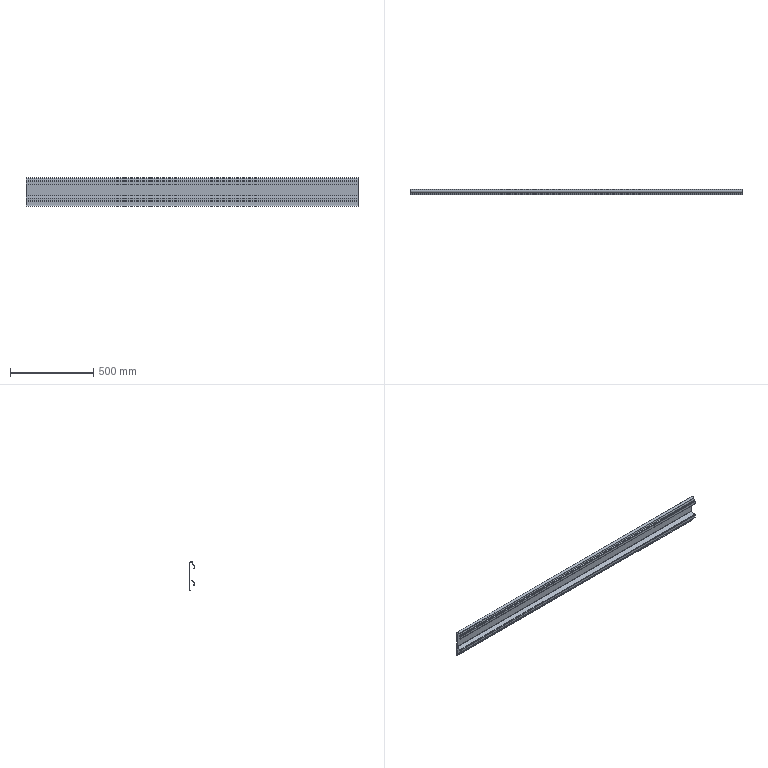Part | NX | features DATUM_CSYS 2, EXTRUDE 1, SKETCH 1 | 1 solid | 45 faces | box 2000 x 29.98 x 174.62 mm | volume 1173848 mm3 | plane 25 | cylinder 20 | commonest cylinder face diameters 1 x14 4 x4 15.24 x1 19.24 x1
STEP:
#1=CARTESIAN_POINT('',(-1000.,0.,-101.016));
#2=VERTEX_POINT('',#1);
#3=CARTESIAN_POINT('',(-1000.,0.,-116.763));
#4=VERTEX_POINT('',#3);
#5=CARTESIAN_POINT('',(-1000.,0.,-101.016));
#6=DIRECTION('',(0.,0.,-1.));
#7=VECTOR('',#6,1000.);
#8=LINE('',#5,#7);
#9=EDGE_CURVE('',#2,#4,#8,.T.);
#10=ORIENTED_EDGE('',*,*,#9,.T.);
#11=CARTESIAN_POINT('',(1000.,0.,-116.763));
#12=VERTEX_POINT('',#11);
#13=CARTESIAN_POINT('',(1000.,0.,-116.763));
#14=DIRECTION('',(-1.,0.,0.));
#15=VECTOR('',#14,1000.);
#16=LINE('',#13,#15);
#17=EDGE_CURVE('',#12,#4,#16,.T.);
#18=ORIENTED_EDGE('',*,*,#17,.F.);
#19=CARTESIAN_POINT('',(1000.,0.,-101.016));
#20=VERTEX_POINT('',#19);
#21=CARTESIAN_POINT('',(1000.,0.,-101.016));
#22=DIRECTION('',(0.,0.,-1.));
#23=VECTOR('',#22,1000.);
#24=LINE('',#21,#23);
#25=EDGE_CURVE('',#20,#12,#24,.T.);
#26=ORIENTED_EDGE('',*,*,#25,.F.);
#27=CARTESIAN_POINT('',(1000.,0.,-101.016));
#28=DIRECTION('',(-1.,0.,0.));
#29=VECTOR('',#28,1000.);
#30=LINE('',#27,#29);
#31=EDGE_CURVE('',#20,#2,#30,.T.);
#32=ORIENTED_EDGE('',*,*,#31,.T.);
#33=EDGE_LOOP('',(#10,#18,#26,#32));
#34=FACE_BOUND('',#33,.T.);
#35=CARTESIAN_POINT('',(1000.,0.,-101.016));
#36=DIRECTION('',(0.,1.,0.));
#37=DIRECTION('',(0.,0.,1.));
#38=AXIS2_PLACEMENT_3D('',#35,#36,#37);
#39=PLANE('',#38);
#40=ADVANCED_FACE('',(#34),#39,.F.);
#41=CARTESIAN_POINT('',(-1000.,2.,-118.763));
#42=VERTEX_POINT('',#41);
#43=CARTESIAN_POINT('',(-1000.,2.,-116.763));
#44=DIRECTION('',(1.,0.,0.));
#45=DIRECTION('',(0.,1.,0.));
#46=AXIS2_PLACEMENT_3D('',#43,#44,#45);
#47=CIRCLE('',#46,2.);
#48=EDGE_CURVE('',#4,#42,#47,.T.);
#49=ORIENTED_EDGE('',*,*,#48,.T.);
#50=CARTESIAN_POINT('',(1000.,2.,-118.763));
#51=VERTEX_POINT('',#50);
#52=CARTESIAN_POINT('',(1000.,2.,-118.763));
#53=DIRECTION('',(-1.,0.,0.));
#54=VECTOR('',#53,1000.);
#55=LINE('',#52,#54);
#56=EDGE_CURVE('',#51,#42,#55,.T.);
#57=ORIENTED_EDGE('',*,*,#56,.F.);
#58=CARTESIAN_POINT('',(1000.,2.,-116.763));
#59=DIRECTION('',(1.,0.,0.));
#60=DIRECTION('',(0.,1.,0.));
#61=AXIS2_PLACEMENT_3D('',#58,#59,#60);
#62=CIRCLE('',#61,2.);
#63=EDGE_CURVE('',#12,#51,#62,.T.);
#64=ORIENTED_EDGE('',*,*,#63,.F.);
#65=ORIENTED_EDGE('',*,*,#17,.T.);
#66=EDGE_LOOP('',(#49,#57,#64,#65));
#67=FACE_BOUND('',#66,.T.);
#68=CARTESIAN_POINT('',(1000.,2.,-116.763));
#69=DIRECTION('',(-1.,0.,0.));
#70=DIRECTION('',(0.,0.,1.));
#71=AXIS2_PLACEMENT_3D('',#68,#69,#70);
#72=CYLINDRICAL_SURFACE('',#71,2.);
#73=ADVANCED_FACE('',(#67),#72,.T.);
#74=CARTESIAN_POINT('',(-1000.,3.696,-118.763));
#75=VERTEX_POINT('',#74);
#76=CARTESIAN_POINT('',(-1000.,2.,-118.763));
#77=DIRECTION('',(0.,1.,0.));
#78=VECTOR('',#77,1000.);
#79=LINE('',#76,#78);
#80=EDGE_CURVE('',#42,#75,#79,.T.);
#81=ORIENTED_EDGE('',*,*,#80,.T.);
#82=CARTESIAN_POINT('',(1000.,3.696,-118.763));
#83=VERTEX_POINT('',#82);
#84=CARTESIAN_POINT('',(1000.,3.696,-118.763));
#85=DIRECTION('',(-1.,0.,0.));
#86=VECTOR('',#85,1000.);
#87=LINE('',#84,#86);
#88=EDGE_CURVE('',#83,#75,#87,.T.);
#89=ORIENTED_EDGE('',*,*,#88,.F.);
#90=CARTESIAN_POINT('',(1000.,2.,-118.763));
#91=DIRECTION('',(0.,1.,0.));
#92=VECTOR('',#91,1000.);
#93=LINE('',#90,#92);
#94=EDGE_CURVE('',#51,#83,#93,.T.);
#95=ORIENTED_EDGE('',*,*,#94,.F.);
#96=ORIENTED_EDGE('',*,*,#56,.T.);
#97=EDGE_LOOP('',(#81,#89,#95,#96));
#98=FACE_BOUND('',#97,.T.);
#99=CARTESIAN_POINT('',(1000.,2.,-118.763));
#100=DIRECTION('',(0.,0.,1.));
#101=DIRECTION('',(1.,0.,0.));
#102=AXIS2_PLACEMENT_3D('',#99,#100,#101);
#103=PLANE('',#102);
#104=ADVANCED_FACE('',(#98),#103,.F.);
#105=CARTESIAN_POINT('',(-1000.,5.581,-117.429));
#106=VERTEX_POINT('',#105);
#107=CARTESIAN_POINT('',(-1000.,3.696,-116.763));
#108=DIRECTION('',(1.,0.,0.));
#109=DIRECTION('',(0.,1.,0.));
#110=AXIS2_PLACEMENT_3D('',#107,#108,#109);
#111=CIRCLE('',#110,2.);
#112=EDGE_CURVE('',#75,#106,#111,.T.);
#113=ORIENTED_EDGE('',*,*,#112,.T.);
#114=CARTESIAN_POINT('',(1000.,5.581,-117.429));
#115=VERTEX_POINT('',#114);
#116=CARTESIAN_POINT('',(1000.,5.581,-117.429));
#117=DIRECTION('',(-1.,0.,0.));
#118=VECTOR('',#117,1000.);
#119=LINE('',#116,#118);
#120=EDGE_CURVE('',#115,#106,#119,.T.);
#121=ORIENTED_EDGE('',*,*,#120,.F.);
#122=CARTESIAN_POINT('',(1000.,3.696,-116.763));
#123=DIRECTION('',(1.,0.,0.));
#124=DIRECTION('',(0.,1.,0.));
#125=AXIS2_PLACEMENT_3D('',#122,#123,#124);
#126=CIRCLE('',#125,2.);
#127=EDGE_CURVE('',#83,#115,#126,.T.);
#128=ORIENTED_EDGE('',*,*,#127,.F.);
#129=ORIENTED_EDGE('',*,*,#88,.T.);
#130=EDGE_LOOP('',(#113,#121,#128,#129));
#131=FACE_BOUND('',#130,.T.);
#132=CARTESIAN_POINT('',(1000.,3.696,-116.763));
#133=DIRECTION('',(-1.,0.,0.));
#134=DIRECTION('',(0.,0.,1.));
#135=AXIS2_PLACEMENT_3D('',#132,#133,#134);
#136=CYLINDRICAL_SURFACE('',#135,2.);
#137=ADVANCED_FACE('',(#131),#136,.T.);
#138=CARTESIAN_POINT('',(-1000.,5.11,-116.763));
#139=VERTEX_POINT('',#138);
#140=CARTESIAN_POINT('',(-1000.,5.11,-117.263));
#141=DIRECTION('',(1.,0.,0.));
#142=DIRECTION('',(0.,1.,0.));
#143=AXIS2_PLACEMENT_3D('',#140,#141,#142);
#144=CIRCLE('',#143,0.5);
#145=EDGE_CURVE('',#106,#139,#144,.T.);
#146=ORIENTED_EDGE('',*,*,#145,.T.);
#147=CARTESIAN_POINT('',(1000.,5.11,-116.763));
#148=VERTEX_POINT('',#147);
#149=CARTESIAN_POINT('',(1000.,5.11,-116.763));
#150=DIRECTION('',(-1.,0.,0.));
#151=VECTOR('',#150,1000.);
#152=LINE('',#149,#151);
#153=EDGE_CURVE('',#148,#139,#152,.T.);
#154=ORIENTED_EDGE('',*,*,#153,.F.);
#155=CARTESIAN_POINT('',(1000.,5.11,-117.263));
#156=DIRECTION('',(1.,0.,0.));
#157=DIRECTION('',(0.,1.,0.));
#158=AXIS2_PLACEMENT_3D('',#155,#156,#157);
#159=CIRCLE('',#158,0.5);
#160=EDGE_CURVE('',#115,#148,#159,.T.);
#161=ORIENTED_EDGE('',*,*,#160,.F.);
#162=ORIENTED_EDGE('',*,*,#120,.T.);
#163=EDGE_LOOP('',(#146,#154,#161,#162));
#164=FACE_BOUND('',#163,.T.);
#165=CARTESIAN_POINT('',(1000.,5.11,-117.263));
#166=DIRECTION('',(-1.,0.,0.));
#167=DIRECTION('',(0.,0.,1.));
#168=AXIS2_PLACEMENT_3D('',#165,#166,#167);
#169=CYLINDRICAL_SURFACE('',#168,0.5);
#170=ADVANCED_FACE('',(#164),#169,.T.);
#171=CARTESIAN_POINT('',(-1000.,2.5,-116.763));
#172=VERTEX_POINT('',#171);
#173=CARTESIAN_POINT('',(-1000.,5.11,-116.763));
#174=DIRECTION('',(0.,-1.,0.));
#175=VECTOR('',#174,1000.);
#176=LINE('',#173,#175);
#177=EDGE_CURVE('',#139,#172,#176,.T.);
#178=ORIENTED_EDGE('',*,*,#177,.T.);
#179=CARTESIAN_POINT('',(1000.,2.5,-116.763));
#180=VERTEX_POINT('',#179);
#181=CARTESIAN_POINT('',(1000.,2.5,-116.763));
#182=DIRECTION('',(-1.,0.,0.));
#183=VECTOR('',#182,1000.);
#184=LINE('',#181,#183);
#185=EDGE_CURVE('',#180,#172,#184,.T.);
#186=ORIENTED_EDGE('',*,*,#185,.F.);
#187=CARTESIAN_POINT('',(1000.,5.11,-116.763));
#188=DIRECTION('',(0.,-1.,0.));
#189=VECTOR('',#188,1000.);
#190=LINE('',#187,#189);
#191=EDGE_CURVE('',#148,#180,#190,.T.);
#192=ORIENTED_EDGE('',*,*,#191,.F.);
#193=ORIENTED_EDGE('',*,*,#153,.T.);
#194=EDGE_LOOP('',(#178,#186,#192,#193));
#195=FACE_BOUND('',#194,.T.);
#196=CARTESIAN_POINT('',(1000.,5.11,-116.763));
#197=DIRECTION('',(0.,0.,-1.));
#198=DIRECTION('',(-1.,0.,0.));
#199=AXIS2_PLACEMENT_3D('',#196,#197,#198);
#200=PLANE('',#199);
#201=ADVANCED_FACE('',(#195),#200,.F.);
#202=CARTESIAN_POINT('',(-1000.,2.,-116.263));
#203=VERTEX_POINT('',#202);
#204=CARTESIAN_POINT('',(-1000.,2.5,-116.263));
#205=DIRECTION('',(-1.,0.,0.));
#206=DIRECTION('',(0.,1.,0.));
#207=AXIS2_PLACEMENT_3D('',#204,#205,#206);
#208=CIRCLE('',#207,0.5);
#209=EDGE_CURVE('',#172,#203,#208,.T.);
#210=ORIENTED_EDGE('',*,*,#209,.T.);
#211=CARTESIAN_POINT('',(1000.,2.,-116.263));
#212=VERTEX_POINT('',#211);
#213=CARTESIAN_POINT('',(1000.,2.,-116.263));
#214=DIRECTION('',(-1.,0.,0.));
#215=VECTOR('',#214,1000.);
#216=LINE('',#213,#215);
#217=EDGE_CURVE('',#212,#203,#216,.T.);
#218=ORIENTED_EDGE('',*,*,#217,.F.);
#219=CARTESIAN_POINT('',(1000.,2.5,-116.263));
#220=DIRECTION('',(-1.,0.,0.));
#221=DIRECTION('',(0.,1.,0.));
#222=AXIS2_PLACEMENT_3D('',#219,#220,#221);
#223=CIRCLE('',#222,0.5);
#224=EDGE_CURVE('',#180,#212,#223,.T.);
#225=ORIENTED_EDGE('',*,*,#224,.F.);
#226=ORIENTED_EDGE('',*,*,#185,.T.);
#227=EDGE_LOOP('',(#210,#218,#225,#226));
#228=FACE_BOUND('',#227,.T.);
#229=CARTESIAN_POINT('',(1000.,2.5,-116.263));
#230=DIRECTION('',(-1.,0.,0.));
#231=DIRECTION('',(0.,0.,1.));
#232=AXIS2_PLACEMENT_3D('',#229,#230,#231);
#233=CYLINDRICAL_SURFACE('',#232,0.5);
#234=ADVANCED_FACE('',(#228),#233,.F.);
#235=CARTESIAN_POINT('',(-1000.,2.,-103.123));
#236=VERTEX_POINT('',#235);
#237=CARTESIAN_POINT('',(-1000.,2.,-116.263));
#238=DIRECTION('',(0.,0.,1.));
#239=VECTOR('',#238,1000.);
#240=LINE('',#237,#239);
#241=EDGE_CURVE('',#203,#236,#240,.T.);
#242=ORIENTED_EDGE('',*,*,#241,.T.);
#243=CARTESIAN_POINT('',(1000.,2.,-103.123));
#244=VERTEX_POINT('',#243);
#245=CARTESIAN_POINT('',(1000.,2.,-103.123));
#246=DIRECTION('',(-1.,0.,0.));
#247=VECTOR('',#246,1000.);
#248=LINE('',#245,#247);
#249=EDGE_CURVE('',#244,#236,#248,.T.);
#250=ORIENTED_EDGE('',*,*,#249,.F.);
#251=CARTESIAN_POINT('',(1000.,2.,-116.263));
#252=DIRECTION('',(0.,0.,1.));
#253=VECTOR('',#252,1000.);
#254=LINE('',#251,#253);
#255=EDGE_CURVE('',#212,#244,#254,.T.);
#256=ORIENTED_EDGE('',*,*,#255,.F.);
#257=ORIENTED_EDGE('',*,*,#217,.T.);
#258=EDGE_LOOP('',(#242,#250,#256,#257));
#259=FACE_BOUND('',#258,.T.);
#260=CARTESIAN_POINT('',(1000.,2.,-116.263));
#261=DIRECTION('',(0.,-1.,0.));
#262=DIRECTION('',(0.,0.,-1.));
#263=AXIS2_PLACEMENT_3D('',#260,#261,#262);
#264=PLANE('',#263);
#265=ADVANCED_FACE('',(#259),#264,.F.);
#266=CARTESIAN_POINT('',(-1000.,2.5,-102.623));
#267=VERTEX_POINT('',#266);
#268=CARTESIAN_POINT('',(-1000.,2.5,-103.123));
#269=DIRECTION('',(-1.,0.,0.));
#270=DIRECTION('',(0.,1.,0.));
#271=AXIS2_PLACEMENT_3D('',#268,#269,#270);
#272=CIRCLE('',#271,0.5);
#273=EDGE_CURVE('',#236,#267,#272,.T.);
#274=ORIENTED_EDGE('',*,*,#273,.T.);
#275=CARTESIAN_POINT('',(1000.,2.5,-102.623));
#276=VERTEX_POINT('',#275);
#277=CARTESIAN_POINT('',(1000.,2.5,-102.623));
#278=DIRECTION('',(-1.,0.,0.));
#279=VECTOR('',#278,1000.);
#280=LINE('',#277,#279);
#281=EDGE_CURVE('',#276,#267,#280,.T.);
#282=ORIENTED_EDGE('',*,*,#281,.F.);
#283=CARTESIAN_POINT('',(1000.,2.5,-103.123));
#284=DIRECTION('',(-1.,0.,0.));
#285=DIRECTION('',(0.,1.,0.));
#286=AXIS2_PLACEMENT_3D('',#283,#284,#285);
#287=CIRCLE('',#286,0.5);
#288=EDGE_CURVE('',#244,#276,#287,.T.);
#289=ORIENTED_EDGE('',*,*,#288,.F.);
#290=ORIENTED_EDGE('',*,*,#249,.T.);
#291=EDGE_LOOP('',(#274,#282,#289,#290));
#292=FACE_BOUND('',#291,.T.);
#293=CARTESIAN_POINT('',(1000.,2.5,-103.123));
#294=DIRECTION('',(-1.,0.,0.));
#295=DIRECTION('',(0.,0.,1.));
#296=AXIS2_PLACEMENT_3D('',#293,#294,#295);
#297=CYLINDRICAL_SURFACE('',#296,0.5);
#298=ADVANCED_FACE('',(#292),#297,.F.);
#299=CARTESIAN_POINT('',(-1000.,4.8,-102.623));
#300=VERTEX_POINT('',#299);
#301=CARTESIAN_POINT('',(-1000.,2.5,-102.623));
#302=DIRECTION('',(0.,1.,0.));
#303=VECTOR('',#302,1000.);
#304=LINE('',#301,#303);
#305=EDGE_CURVE('',#267,#300,#304,.T.);
#306=ORIENTED_EDGE('',*,*,#305,.T.);
#307=CARTESIAN_POINT('',(1000.,4.8,-102.623));
#308=VERTEX_POINT('',#307);
#309=CARTESIAN_POINT('',(1000.,4.8,-102.623));
#310=DIRECTION('',(-1.,0.,0.));
#311=VECTOR('',#310,1000.);
#312=LINE('',#309,#311);
#313=EDGE_CURVE('',#308,#300,#312,.T.);
#314=ORIENTED_EDGE('',*,*,#313,.F.);
#315=CARTESIAN_POINT('',(1000.,2.5,-102.623));
#316=DIRECTION('',(0.,1.,0.));
#317=VECTOR('',#316,1000.);
#318=LINE('',#315,#317);
#319=EDGE_CURVE('',#276,#308,#318,.T.);
#320=ORIENTED_EDGE('',*,*,#319,.F.);
#321=ORIENTED_EDGE('',*,*,#281,.T.);
#322=EDGE_LOOP('',(#306,#314,#320,#321));
#323=FACE_BOUND('',#322,.T.);
#324=CARTESIAN_POINT('',(1000.,2.5,-102.623));
#325=DIRECTION('',(0.,0.,1.));
#326=DIRECTION('',(1.,0.,0.));
#327=AXIS2_PLACEMENT_3D('',#324,#325,#326);
#328=PLANE('',#327);
#329=ADVANCED_FACE('',(#323),#328,.F.);
#330=CARTESIAN_POINT('',(-1000.,5.3,-102.123));
#331=VERTEX_POINT('',#330);
#332=CARTESIAN_POINT('',(-1000.,4.8,-102.123));
#333=DIRECTION('',(1.,0.,0.));
#334=DIRECTION('',(0.,1.,0.));
#335=AXIS2_PLACEMENT_3D('',#332,#333,#334);
#336=CIRCLE('',#335,0.5);
#337=EDGE_CURVE('',#300,#331,#336,.T.);
#338=ORIENTED_EDGE('',*,*,#337,.T.);
#339=CARTESIAN_POINT('',(1000.,5.3,-102.123));
#340=VERTEX_POINT('',#339);
#341=CARTESIAN_POINT('',(1000.,5.3,-102.123));
#342=DIRECTION('',(-1.,0.,0.));
#343=VECTOR('',#342,1000.);
#344=LINE('',#341,#343);
#345=EDGE_CURVE('',#340,#331,#344,.T.);
#346=ORIENTED_EDGE('',*,*,#345,.F.);
#347=CARTESIAN_POINT('',(1000.,4.8,-102.123));
#348=DIRECTION('',(1.,0.,0.));
#349=DIRECTION('',(0.,1.,0.));
#350=AXIS2_PLACEMENT_3D('',#347,#348,#349);
#351=CIRCLE('',#350,0.5);
#352=EDGE_CURVE('',#308,#340,#351,.T.);
#353=ORIENTED_EDGE('',*,*,#352,.F.);
#354=ORIENTED_EDGE('',*,*,#313,.T.);
#355=EDGE_LOOP('',(#338,#346,#353,#354));
#356=FACE_BOUND('',#355,.T.);
#357=CARTESIAN_POINT('',(1000.,4.8,-102.123));
#358=DIRECTION('',(-1.,0.,0.));
#359=DIRECTION('',(0.,0.,1.));
#360=AXIS2_PLACEMENT_3D('',#357,#358,#359);
#361=CYLINDRICAL_SURFACE('',#360,0.5);
#362=ADVANCED_FACE('',(#356),#361,.T.);
#363=CARTESIAN_POINT('',(-1000.,5.3,-100.463));
#364=VERTEX_POINT('',#363);
#365=CARTESIAN_POINT('',(-1000.,5.3,-102.123));
#366=DIRECTION('',(0.,0.,1.));
#367=VECTOR('',#366,1000.);
#368=LINE('',#365,#367);
#369=EDGE_CURVE('',#331,#364,#368,.T.);
#370=ORIENTED_EDGE('',*,*,#369,.T.);
#371=CARTESIAN_POINT('',(1000.,5.3,-100.463));
#372=VERTEX_POINT('',#371);
#373=CARTESIAN_POINT('',(1000.,5.3,-100.463));
#374=DIRECTION('',(-1.,0.,0.));
#375=VECTOR('',#374,1000.);
#376=LINE('',#373,#375);
#377=EDGE_CURVE('',#372,#364,#376,.T.);
#378=ORIENTED_EDGE('',*,*,#377,.F.);
#379=CARTESIAN_POINT('',(1000.,5.3,-102.123));
#380=DIRECTION('',(0.,0.,1.));
#381=VECTOR('',#380,1000.);
#382=LINE('',#379,#381);
#383=EDGE_CURVE('',#340,#372,#382,.T.);
#384=ORIENTED_EDGE('',*,*,#383,.F.);
#385=ORIENTED_EDGE('',*,*,#345,.T.);
#386=EDGE_LOOP('',(#370,#378,#384,#385));
#387=FACE_BOUND('',#386,.T.);
#388=CARTESIAN_POINT('',(1000.,5.3,-102.123));
#389=DIRECTION('',(0.,-1.,0.));
#390=DIRECTION('',(0.,0.,-1.));
#391=AXIS2_PLACEMENT_3D('',#388,#389,#390);
#392=PLANE('',#391);
#393=ADVANCED_FACE('',(#387),#392,.F.);
#394=CARTESIAN_POINT('',(-1000.,5.565,-100.021));
#395=VERTEX_POINT('',#394);
#396=CARTESIAN_POINT('',(-1000.,5.8,-100.463));
#397=DIRECTION('',(-1.,0.,0.));
#398=DIRECTION('',(0.,1.,0.));
#399=AXIS2_PLACEMENT_3D('',#396,#397,#398);
#400=CIRCLE('',#399,0.5);
#401=EDGE_CURVE('',#364,#395,#400,.T.);
#402=ORIENTED_EDGE('',*,*,#401,.T.);
#403=CARTESIAN_POINT('',(1000.,5.565,-100.021));
#404=VERTEX_POINT('',#403);
#405=CARTESIAN_POINT('',(1000.,5.565,-100.021));
#406=DIRECTION('',(-1.,0.,0.));
#407=VECTOR('',#406,1000.);
#408=LINE('',#405,#407);
#409=EDGE_CURVE('',#404,#395,#408,.T.);
#410=ORIENTED_EDGE('',*,*,#409,.F.);
#411=CARTESIAN_POINT('',(1000.,5.8,-100.463));
#412=DIRECTION('',(-1.,0.,0.));
#413=DIRECTION('',(0.,1.,0.));
#414=AXIS2_PLACEMENT_3D('',#411,#412,#413);
#415=CIRCLE('',#414,0.5);
#416=EDGE_CURVE('',#372,#404,#415,.T.);
#417=ORIENTED_EDGE('',*,*,#416,.F.);
#418=ORIENTED_EDGE('',*,*,#377,.T.);
#419=EDGE_LOOP('',(#402,#410,#417,#418));
#420=FACE_BOUND('',#419,.T.);
#421=CARTESIAN_POINT('',(1000.,5.8,-100.463));
#422=DIRECTION('',(-1.,0.,0.));
#423=DIRECTION('',(0.,0.,1.));
#424=AXIS2_PLACEMENT_3D('',#421,#422,#423);
#425=CYLINDRICAL_SURFACE('',#424,0.5);
#426=ADVANCED_FACE('',(#420),#425,.F.);
#427=CARTESIAN_POINT('',(-1000.,27.98,-88.103));
#428=VERTEX_POINT('',#427);
#429=CARTESIAN_POINT('',(-1000.,5.565,-100.021));
#430=DIRECTION('',(0.,0.8829,0.4695));
#431=VECTOR('',#430,1000.);
#432=LINE('',#429,#431);
#433=EDGE_CURVE('',#395,#428,#432,.T.);
#434=ORIENTED_EDGE('',*,*,#433,.T.);
#435=CARTESIAN_POINT('',(1000.,27.98,-88.103));
#436=VERTEX_POINT('',#435);
#437=CARTESIAN_POINT('',(1000.,27.98,-88.103));
#438=DIRECTION('',(-1.,0.,0.));
#439=VECTOR('',#438,1000.);
#440=LINE('',#437,#439);
#441=EDGE_CURVE('',#436,#428,#440,.T.);
#442=ORIENTED_EDGE('',*,*,#441,.F.);
#443=CARTESIAN_POINT('',(1000.,5.565,-100.021));
#444=DIRECTION('',(0.,0.8829,0.4695));
#445=VECTOR('',#444,1000.);
#446=LINE('',#443,#445);
#447=EDGE_CURVE('',#404,#436,#446,.T.);
#448=ORIENTED_EDGE('',*,*,#447,.F.);
#449=ORIENTED_EDGE('',*,*,#409,.T.);
#450=EDGE_LOOP('',(#434,#442,#448,#449));
#451=FACE_BOUND('',#450,.T.);
#452=CARTESIAN_POINT('',(1000.,5.565,-100.021));
#453=DIRECTION('',(0.,-0.4695,0.8829));
#454=DIRECTION('',(0.,-0.8829,-0.4695));
#455=AXIS2_PLACEMENT_3D('',#452,#453,#454);
#456=PLANE('',#455);
#457=ADVANCED_FACE('',(#451),#456,.F.);
#458=CARTESIAN_POINT('',(-1000.,27.98,-144.348));
#459=VERTEX_POINT('',#458);
#460=CARTESIAN_POINT('',(-1000.,27.98,-88.103));
#461=DIRECTION('',(0.,0.,-1.));
#462=VECTOR('',#461,1000.);
#463=LINE('',#460,#462);
#464=EDGE_CURVE('',#428,#459,#463,.T.);
#465=ORIENTED_EDGE('',*,*,#464,.T.);
#466=CARTESIAN_POINT('',(1000.,27.98,-144.348));
#467=VERTEX_POINT('',#466);
#468=CARTESIAN_POINT('',(1000.,27.98,-144.348));
#469=DIRECTION('',(-1.,0.,0.));
#470=VECTOR('',#469,1000.);
#471=LINE('',#468,#470);
#472=EDGE_CURVE('',#467,#459,#471,.T.);
#473=ORIENTED_EDGE('',*,*,#472,.F.);
#474=CARTESIAN_POINT('',(1000.,27.98,-88.103));
#475=DIRECTION('',(0.,0.,-1.));
#476=VECTOR('',#475,1000.);
#477=LINE('',#474,#476);
#478=EDGE_CURVE('',#436,#467,#477,.T.);
#479=ORIENTED_EDGE('',*,*,#478,.F.);
#480=ORIENTED_EDGE('',*,*,#441,.T.);
#481=EDGE_LOOP('',(#465,#473,#479,#480));
#482=FACE_BOUND('',#481,.T.);
#483=CARTESIAN_POINT('',(1000.,27.98,-88.103));
#484=DIRECTION('',(0.,1.,0.));
#485=DIRECTION('',(0.,0.,1.));
#486=AXIS2_PLACEMENT_3D('',#483,#484,#485);
#487=PLANE('',#486);
#488=ADVANCED_FACE('',(#482),#487,.F.);
#489=CARTESIAN_POINT('',(-1000.,25.215,-150.359));
#490=VERTEX_POINT('',#489);
#491=CARTESIAN_POINT('',(-1000.,27.98,-144.348));
#492=DIRECTION('',(0.,-0.4179,-0.9085));
#493=VECTOR('',#492,1000.);
#494=LINE('',#491,#493);
#495=EDGE_CURVE('',#459,#490,#494,.T.);
#496=ORIENTED_EDGE('',*,*,#495,.T.);
#497=CARTESIAN_POINT('',(1000.,25.215,-150.359));
#498=VERTEX_POINT('',#497);
#499=CARTESIAN_POINT('',(1000.,25.215,-150.359));
#500=DIRECTION('',(-1.,0.,0.));
#501=VECTOR('',#500,1000.);
#502=LINE('',#499,#501);
#503=EDGE_CURVE('',#498,#490,#502,.T.);
#504=ORIENTED_EDGE('',*,*,#503,.F.);
#505=CARTESIAN_POINT('',(1000.,27.98,-144.348));
#506=DIRECTION('',(0.,-0.4179,-0.9085));
#507=VECTOR('',#506,1000.);
#508=LINE('',#505,#507);
#509=EDGE_CURVE('',#467,#498,#508,.T.);
#510=ORIENTED_EDGE('',*,*,#509,.F.);
#511=ORIENTED_EDGE('',*,*,#472,.T.);
#512=EDGE_LOOP('',(#496,#504,#510,#511));
#513=FACE_BOUND('',#512,.T.);
#514=CARTESIAN_POINT('',(1000.,27.98,-144.348));
#515=DIRECTION('',(0.,0.9085,-0.4179));
#516=DIRECTION('',(0.,0.4179,0.9085));
#517=AXIS2_PLACEMENT_3D('',#514,#515,#516);
#518=PLANE('',#517);
#519=ADVANCED_FACE('',(#513),#518,.F.);
#520=CARTESIAN_POINT('',(-1000.,25.669,-151.068));
#521=VERTEX_POINT('',#520);
#522=CARTESIAN_POINT('',(-1000.,25.669,-150.568));
#523=DIRECTION('',(1.,0.,0.));
#524=DIRECTION('',(0.,1.,0.));
#525=AXIS2_PLACEMENT_3D('',#522,#523,#524);
#526=CIRCLE('',#525,0.5);
#527=EDGE_CURVE('',#490,#521,#526,.T.);
#528=ORIENTED_EDGE('',*,*,#527,.T.);
#529=CARTESIAN_POINT('',(1000.,25.669,-151.068));
#530=VERTEX_POINT('',#529);
#531=CARTESIAN_POINT('',(1000.,25.669,-151.068));
#532=DIRECTION('',(-1.,0.,0.));
#533=VECTOR('',#532,1000.);
#534=LINE('',#531,#533);
#535=EDGE_CURVE('',#530,#521,#534,.T.);
#536=ORIENTED_EDGE('',*,*,#535,.F.);
#537=CARTESIAN_POINT('',(1000.,25.669,-150.568));
#538=DIRECTION('',(1.,0.,0.));
#539=DIRECTION('',(0.,1.,0.));
#540=AXIS2_PLACEMENT_3D('',#537,#538,#539);
#541=CIRCLE('',#540,0.5);
#542=EDGE_CURVE('',#498,#530,#541,.T.);
#543=ORIENTED_EDGE('',*,*,#542,.F.);
#544=ORIENTED_EDGE('',*,*,#503,.T.);
#545=EDGE_LOOP('',(#528,#536,#543,#544));
#546=FACE_BOUND('',#545,.T.);
#547=CARTESIAN_POINT('',(1000.,25.669,-150.568));
#548=DIRECTION('',(-1.,0.,0.));
#549=DIRECTION('',(0.,0.,1.));
#550=AXIS2_PLACEMENT_3D('',#547,#548,#549);
#551=CYLINDRICAL_SURFACE('',#550,0.5);
#552=ADVANCED_FACE('',(#546),#551,.T.);
#553=CARTESIAN_POINT('',(-1000.,29.98,-151.068));
#554=VERTEX_POINT('',#553);
#555=CARTESIAN_POINT('',(-1000.,25.669,-151.068));
#556=DIRECTION('',(0.,1.,0.));
#557=VECTOR('',#556,1000.);
#558=LINE('',#555,#557);
#559=EDGE_CURVE('',#521,#554,#558,.T.);
#560=ORIENTED_EDGE('',*,*,#559,.T.);
#561=CARTESIAN_POINT('',(1000.,29.98,-151.068));
#562=VERTEX_POINT('',#561);
#563=CARTESIAN_POINT('',(1000.,29.98,-151.068));
#564=DIRECTION('',(-1.,0.,0.));
#565=VECTOR('',#564,1000.);
#566=LINE('',#563,#565);
#567=EDGE_CURVE('',#562,#554,#566,.T.);
#568=ORIENTED_EDGE('',*,*,#567,.F.);
#569=CARTESIAN_POINT('',(1000.,25.669,-151.068));
#570=DIRECTION('',(0.,1.,0.));
#571=VECTOR('',#570,1000.);
#572=LINE('',#569,#571);
#573=EDGE_CURVE('',#530,#562,#572,.T.);
#574=ORIENTED_EDGE('',*,*,#573,.F.);
#575=ORIENTED_EDGE('',*,*,#535,.T.);
#576=EDGE_LOOP('',(#560,#568,#574,#575));
#577=FACE_BOUND('',#576,.T.);
#578=CARTESIAN_POINT('',(1000.,25.669,-151.068));
#579=DIRECTION('',(0.,0.,1.));
#580=DIRECTION('',(0.,-1.,0.));
#581=AXIS2_PLACEMENT_3D('',#578,#579,#580);
#582=PLANE('',#581);
#583=ADVANCED_FACE('',(#577),#582,.F.);
#584=CARTESIAN_POINT('',(-1000.,29.98,13.932));
#585=VERTEX_POINT('',#584);
#586=CARTESIAN_POINT('',(-1000.,29.98,-151.068));
#587=DIRECTION('',(0.,0.,1.));
#588=VECTOR('',#587,1000.);
#589=LINE('',#586,#588);
#590=EDGE_CURVE('',#554,#585,#589,.T.);
#591=ORIENTED_EDGE('',*,*,#590,.T.);
#592=CARTESIAN_POINT('',(1000.,29.98,13.932));
#593=VERTEX_POINT('',#592);
#594=CARTESIAN_POINT('',(1000.,29.98,13.932));
#595=DIRECTION('',(-1.,0.,0.));
#596=VECTOR('',#595,1000.);
#597=LINE('',#594,#596);
#598=EDGE_CURVE('',#593,#585,#597,.T.);
#599=ORIENTED_EDGE('',*,*,#598,.F.);
#600=CARTESIAN_POINT('',(1000.,29.98,-151.068));
#601=DIRECTION('',(0.,0.,1.));
#602=VECTOR('',#601,1000.);
#603=LINE('',#600,#602);
#604=EDGE_CURVE('',#562,#593,#603,.T.);
#605=ORIENTED_EDGE('',*,*,#604,.F.);
#606=ORIENTED_EDGE('',*,*,#567,.T.);
#607=EDGE_LOOP('',(#591,#599,#605,#606));
#608=FACE_BOUND('',#607,.T.);
#609=CARTESIAN_POINT('',(1000.,29.98,-151.068));
#610=DIRECTION('',(0.,-1.,0.));
#611=DIRECTION('',(0.,0.,-1.));
#612=AXIS2_PLACEMENT_3D('',#609,#610,#611);
#613=PLANE('',#612);
#614=ADVANCED_FACE('',(#608),#613,.F.);
#615=CARTESIAN_POINT('',(-1000.,10.917,15.768));
#616=VERTEX_POINT('',#615);
#617=CARTESIAN_POINT('',(-1000.,20.36,13.932));
#618=DIRECTION('',(1.,0.,0.));
#619=DIRECTION('',(0.,1.,0.));
#620=AXIS2_PLACEMENT_3D('',#617,#618,#619);
#621=CIRCLE('',#620,9.62);
#622=EDGE_CURVE('',#585,#616,#621,.T.);
#623=ORIENTED_EDGE('',*,*,#622,.T.);
#624=CARTESIAN_POINT('',(1000.,10.917,15.768));
#625=VERTEX_POINT('',#624);
#626=CARTESIAN_POINT('',(1000.,10.917,15.768));
#627=DIRECTION('',(-1.,0.,0.));
#628=VECTOR('',#627,1000.);
#629=LINE('',#626,#628);
#630=EDGE_CURVE('',#625,#616,#629,.T.);
#631=ORIENTED_EDGE('',*,*,#630,.F.);
#632=CARTESIAN_POINT('',(1000.,20.36,13.932));
#633=DIRECTION('',(1.,0.,0.));
#634=DIRECTION('',(0.,1.,0.));
#635=AXIS2_PLACEMENT_3D('',#632,#633,#634);
#636=CIRCLE('',#635,9.62);
#637=EDGE_CURVE('',#593,#625,#636,.T.);
#638=ORIENTED_EDGE('',*,*,#637,.F.);
#639=ORIENTED_EDGE('',*,*,#598,.T.);
#640=EDGE_LOOP('',(#623,#631,#638,#639));
#641=FACE_BOUND('',#640,.T.);
#642=CARTESIAN_POINT('',(1000.,20.36,13.932));
#643=DIRECTION('',(-1.,0.,0.));
#644=DIRECTION('',(0.,0.,1.));
#645=AXIS2_PLACEMENT_3D('',#642,#643,#644);
#646=CYLINDRICAL_SURFACE('',#645,9.62);
#647=ADVANCED_FACE('',(#641),#646,.T.);
#648=CARTESIAN_POINT('',(-1000.,8.757,4.656));
#649=VERTEX_POINT('',#648);
#650=CARTESIAN_POINT('',(-1000.,10.917,15.768));
#651=DIRECTION('',(0.,-0.1908,-0.9816));
#652=VECTOR('',#651,1000.);
#653=LINE('',#650,#652);
#654=EDGE_CURVE('',#616,#649,#653,.T.);
#655=ORIENTED_EDGE('',*,*,#654,.T.);
#656=CARTESIAN_POINT('',(1000.,8.757,4.656));
#657=VERTEX_POINT('',#656);
#658=CARTESIAN_POINT('',(1000.,8.757,4.656));
#659=DIRECTION('',(-1.,0.,0.));
#660=VECTOR('',#659,1000.);
#661=LINE('',#658,#660);
#662=EDGE_CURVE('',#657,#649,#661,.T.);
#663=ORIENTED_EDGE('',*,*,#662,.F.);
#664=CARTESIAN_POINT('',(1000.,10.917,15.768));
#665=DIRECTION('',(0.,-0.1908,-0.9816));
#666=VECTOR('',#665,1000.);
#667=LINE('',#664,#666);
#668=EDGE_CURVE('',#625,#657,#667,.T.);
#669=ORIENTED_EDGE('',*,*,#668,.F.);
#670=ORIENTED_EDGE('',*,*,#630,.T.);
#671=EDGE_LOOP('',(#655,#663,#669,#670));
#672=FACE_BOUND('',#671,.T.);
#673=CARTESIAN_POINT('',(1000.,10.917,15.768));
#674=DIRECTION('',(0.,0.9816,-0.1908));
#675=DIRECTION('',(0.,0.1908,0.9816));
#676=AXIS2_PLACEMENT_3D('',#673,#674,#675);
#677=PLANE('',#676);
#678=ADVANCED_FACE('',(#672),#677,.F.);
#679=CARTESIAN_POINT('',(-1000.,0.2653,0.141));
#680=VERTEX_POINT('',#679);
#681=CARTESIAN_POINT('',(-1000.,8.757,4.656));
#682=DIRECTION('',(0.,-0.8829,-0.4695));
#683=VECTOR('',#682,1000.);
#684=LINE('',#681,#683);
#685=EDGE_CURVE('',#649,#680,#684,.T.);
#686=ORIENTED_EDGE('',*,*,#685,.T.);
#687=CARTESIAN_POINT('',(1000.,0.2653,0.141));
#688=VERTEX_POINT('',#687);
#689=CARTESIAN_POINT('',(1000.,0.2653,0.141));
#690=DIRECTION('',(-1.,0.,0.));
#691=VECTOR('',#690,1000.);
#692=LINE('',#689,#691);
#693=EDGE_CURVE('',#688,#680,#692,.T.);
#694=ORIENTED_EDGE('',*,*,#693,.F.);
#695=CARTESIAN_POINT('',(1000.,8.757,4.656));
#696=DIRECTION('',(0.,-0.8829,-0.4695));
#697=VECTOR('',#696,1000.);
#698=LINE('',#695,#697);
#699=EDGE_CURVE('',#657,#688,#698,.T.);
#700=ORIENTED_EDGE('',*,*,#699,.F.);
#701=ORIENTED_EDGE('',*,*,#662,.T.);
#702=EDGE_LOOP('',(#686,#694,#700,#701));
#703=FACE_BOUND('',#702,.T.);
#704=CARTESIAN_POINT('',(1000.,8.757,4.656));
#705=DIRECTION('',(0.,0.4695,-0.8829));
#706=DIRECTION('',(0.,0.8829,0.4695));
#707=AXIS2_PLACEMENT_3D('',#704,#705,#706);
#708=PLANE('',#707);
#709=ADVANCED_FACE('',(#703),#708,.F.);
#710=CARTESIAN_POINT('',(-1000.,0.,-0.3004));
#711=VERTEX_POINT('',#710);
#712=CARTESIAN_POINT('',(-1000.,0.5,-0.3004));
#713=DIRECTION('',(1.,0.,0.));
#714=DIRECTION('',(0.,1.,0.));
#715=AXIS2_PLACEMENT_3D('',#712,#713,#714);
#716=CIRCLE('',#715,0.5);
#717=EDGE_CURVE('',#680,#711,#716,.T.);
#718=ORIENTED_EDGE('',*,*,#717,.T.);
#719=CARTESIAN_POINT('',(1000.,0.,-0.3004));
#720=VERTEX_POINT('',#719);
#721=CARTESIAN_POINT('',(1000.,0.,-0.3004));
#722=DIRECTION('',(-1.,0.,0.));
#723=VECTOR('',#722,1000.);
#724=LINE('',#721,#723);
#725=EDGE_CURVE('',#720,#711,#724,.T.);
#726=ORIENTED_EDGE('',*,*,#725,.F.);
#727=CARTESIAN_POINT('',(1000.,0.5,-0.3004));
#728=DIRECTION('',(1.,0.,0.));
#729=DIRECTION('',(0.,1.,0.));
#730=AXIS2_PLACEMENT_3D('',#727,#728,#729);
#731=CIRCLE('',#730,0.5);
#732=EDGE_CURVE('',#688,#720,#731,.T.);
#733=ORIENTED_EDGE('',*,*,#732,.F.);
#734=ORIENTED_EDGE('',*,*,#693,.T.);
#735=EDGE_LOOP('',(#718,#726,#733,#734));
#736=FACE_BOUND('',#735,.T.);
#737=CARTESIAN_POINT('',(1000.,0.5,-0.3004));
#738=DIRECTION('',(-1.,0.,0.));
#739=DIRECTION('',(0.,0.,1.));
#740=AXIS2_PLACEMENT_3D('',#737,#738,#739);
#741=CYLINDRICAL_SURFACE('',#740,0.5);
#742=ADVANCED_FACE('',(#736),#741,.T.);
#743=CARTESIAN_POINT('',(-1000.,0.,-16.048));
#744=VERTEX_POINT('',#743);
#745=CARTESIAN_POINT('',(-1000.,0.,-0.3004));
#746=DIRECTION('',(0.,0.,-1.));
#747=VECTOR('',#746,1000.);
#748=LINE('',#745,#747);
#749=EDGE_CURVE('',#711,#744,#748,.T.);
#750=ORIENTED_EDGE('',*,*,#749,.T.);
#751=CARTESIAN_POINT('',(1000.,0.,-16.048));
#752=VERTEX_POINT('',#751);
#753=CARTESIAN_POINT('',(1000.,0.,-16.048));
#754=DIRECTION('',(-1.,0.,0.));
#755=VECTOR('',#754,1000.);
#756=LINE('',#753,#755);
#757=EDGE_CURVE('',#752,#744,#756,.T.);
#758=ORIENTED_EDGE('',*,*,#757,.F.);
#759=CARTESIAN_POINT('',(1000.,0.,-0.3004));
#760=DIRECTION('',(0.,0.,-1.));
#761=VECTOR('',#760,1000.);
#762=LINE('',#759,#761);
#763=EDGE_CURVE('',#720,#752,#762,.T.);
#764=ORIENTED_EDGE('',*,*,#763,.F.);
#765=ORIENTED_EDGE('',*,*,#725,.T.);
#766=EDGE_LOOP('',(#750,#758,#764,#765));
#767=FACE_BOUND('',#766,.T.);
#768=CARTESIAN_POINT('',(1000.,0.,-0.3004));
#769=DIRECTION('',(0.,1.,0.));
#770=DIRECTION('',(0.,0.,1.));
#771=AXIS2_PLACEMENT_3D('',#768,#769,#770);
#772=PLANE('',#771);
#773=ADVANCED_FACE('',(#767),#772,.F.);
#774=CARTESIAN_POINT('',(-1000.,2.,-18.048));
#775=VERTEX_POINT('',#774);
#776=CARTESIAN_POINT('',(-1000.,2.,-16.048));
#777=DIRECTION('',(1.,0.,0.));
#778=DIRECTION('',(0.,1.,0.));
#779=AXIS2_PLACEMENT_3D('',#776,#777,#778);
#780=CIRCLE('',#779,2.);
#781=EDGE_CURVE('',#744,#775,#780,.T.);
#782=ORIENTED_EDGE('',*,*,#781,.T.);
#783=CARTESIAN_POINT('',(1000.,2.,-18.048));
#784=VERTEX_POINT('',#783);
#785=CARTESIAN_POINT('',(1000.,2.,-18.048));
#786=DIRECTION('',(-1.,0.,0.));
#787=VECTOR('',#786,1000.);
#788=LINE('',#785,#787);
#789=EDGE_CURVE('',#784,#775,#788,.T.);
#790=ORIENTED_EDGE('',*,*,#789,.F.);
#791=CARTESIAN_POINT('',(1000.,2.,-16.048));
#792=DIRECTION('',(1.,0.,0.));
#793=DIRECTION('',(0.,1.,0.));
#794=AXIS2_PLACEMENT_3D('',#791,#792,#793);
#795=CIRCLE('',#794,2.);
#796=EDGE_CURVE('',#752,#784,#795,.T.);
#797=ORIENTED_EDGE('',*,*,#796,.F.);
#798=ORIENTED_EDGE('',*,*,#757,.T.);
#799=EDGE_LOOP('',(#782,#790,#797,#798));
#800=FACE_BOUND('',#799,.T.);
#801=CARTESIAN_POINT('',(1000.,2.,-16.048));
#802=DIRECTION('',(-1.,0.,0.));
#803=DIRECTION('',(0.,0.,1.));
#804=AXIS2_PLACEMENT_3D('',#801,#802,#803);
#805=CYLINDRICAL_SURFACE('',#804,2.);
#806=ADVANCED_FACE('',(#800),#805,.T.);
#807=CARTESIAN_POINT('',(-1000.,3.696,-18.048));
#808=VERTEX_POINT('',#807);
#809=CARTESIAN_POINT('',(-1000.,2.,-18.048));
#810=DIRECTION('',(0.,1.,0.));
#811=VECTOR('',#810,1000.);
#812=LINE('',#809,#811);
#813=EDGE_CURVE('',#775,#808,#812,.T.);
#814=ORIENTED_EDGE('',*,*,#813,.T.);
#815=CARTESIAN_POINT('',(1000.,3.696,-18.048));
#816=VERTEX_POINT('',#815);
#817=CARTESIAN_POINT('',(1000.,3.696,-18.048));
#818=DIRECTION('',(-1.,0.,0.));
#819=VECTOR('',#818,1000.);
#820=LINE('',#817,#819);
#821=EDGE_CURVE('',#816,#808,#820,.T.);
#822=ORIENTED_EDGE('',*,*,#821,.F.);
#823=CARTESIAN_POINT('',(1000.,2.,-18.048));
#824=DIRECTION('',(0.,1.,0.));
#825=VECTOR('',#824,1000.);
#826=LINE('',#823,#825);
#827=EDGE_CURVE('',#784,#816,#826,.T.);
#828=ORIENTED_EDGE('',*,*,#827,.F.);
#829=ORIENTED_EDGE('',*,*,#789,.T.);
#830=EDGE_LOOP('',(#814,#822,#828,#829));
#831=FACE_BOUND('',#830,.T.);
#832=CARTESIAN_POINT('',(1000.,2.,-18.048));
#833=DIRECTION('',(0.,0.,1.));
#834=DIRECTION('',(0.,-1.,0.));
#835=AXIS2_PLACEMENT_3D('',#832,#833,#834);
#836=PLANE('',#835);
#837=ADVANCED_FACE('',(#831),#836,.F.);
#838=CARTESIAN_POINT('',(-1000.,5.581,-16.714));
#839=VERTEX_POINT('',#838);
#840=CARTESIAN_POINT('',(-1000.,3.696,-16.048));
#841=DIRECTION('',(1.,0.,0.));
#842=DIRECTION('',(0.,1.,0.));
#843=AXIS2_PLACEMENT_3D('',#840,#841,#842);
#844=CIRCLE('',#843,2.);
#845=EDGE_CURVE('',#808,#839,#844,.T.);
#846=ORIENTED_EDGE('',*,*,#845,.T.);
#847=CARTESIAN_POINT('',(1000.,5.581,-16.714));
#848=VERTEX_POINT('',#847);
#849=CARTESIAN_POINT('',(1000.,5.581,-16.714));
#850=DIRECTION('',(-1.,0.,0.));
#851=VECTOR('',#850,1000.);
#852=LINE('',#849,#851);
#853=EDGE_CURVE('',#848,#839,#852,.T.);
#854=ORIENTED_EDGE('',*,*,#853,.F.);
#855=CARTESIAN_POINT('',(1000.,3.696,-16.048));
#856=DIRECTION('',(1.,0.,0.));
#857=DIRECTION('',(0.,1.,0.));
#858=AXIS2_PLACEMENT_3D('',#855,#856,#857);
#859=CIRCLE('',#858,2.);
#860=EDGE_CURVE('',#816,#848,#859,.T.);
#861=ORIENTED_EDGE('',*,*,#860,.F.);
#862=ORIENTED_EDGE('',*,*,#821,.T.);
#863=EDGE_LOOP('',(#846,#854,#861,#862));
#864=FACE_BOUND('',#863,.T.);
#865=CARTESIAN_POINT('',(1000.,3.696,-16.048));
#866=DIRECTION('',(-1.,0.,0.));
#867=DIRECTION('',(0.,0.,1.));
#868=AXIS2_PLACEMENT_3D('',#865,#866,#867);
#869=CYLINDRICAL_SURFACE('',#868,2.);
#870=ADVANCED_FACE('',(#864),#869,.T.);
#871=CARTESIAN_POINT('',(-1000.,5.11,-16.048));
#872=VERTEX_POINT('',#871);
#873=CARTESIAN_POINT('',(-1000.,5.11,-16.548));
#874=DIRECTION('',(1.,0.,0.));
#875=DIRECTION('',(0.,1.,0.));
#876=AXIS2_PLACEMENT_3D('',#873,#874,#875);
#877=CIRCLE('',#876,0.5);
#878=EDGE_CURVE('',#839,#872,#877,.T.);
#879=ORIENTED_EDGE('',*,*,#878,.T.);
#880=CARTESIAN_POINT('',(1000.,5.11,-16.048));
#881=VERTEX_POINT('',#880);
#882=CARTESIAN_POINT('',(1000.,5.11,-16.048));
#883=DIRECTION('',(-1.,0.,0.));
#884=VECTOR('',#883,1000.);
#885=LINE('',#882,#884);
#886=EDGE_CURVE('',#881,#872,#885,.T.);
#887=ORIENTED_EDGE('',*,*,#886,.F.);
#888=CARTESIAN_POINT('',(1000.,5.11,-16.548));
#889=DIRECTION('',(1.,0.,0.));
#890=DIRECTION('',(0.,1.,0.));
#891=AXIS2_PLACEMENT_3D('',#888,#889,#890);
#892=CIRCLE('',#891,0.5);
#893=EDGE_CURVE('',#848,#881,#892,.T.);
#894=ORIENTED_EDGE('',*,*,#893,.F.);
#895=ORIENTED_EDGE('',*,*,#853,.T.);
#896=EDGE_LOOP('',(#879,#887,#894,#895));
#897=FACE_BOUND('',#896,.T.);
#898=CARTESIAN_POINT('',(1000.,5.11,-16.548));
#899=DIRECTION('',(-1.,0.,0.));
#900=DIRECTION('',(0.,0.,1.));
#901=AXIS2_PLACEMENT_3D('',#898,#899,#900);
#902=CYLINDRICAL_SURFACE('',#901,0.5);
#903=ADVANCED_FACE('',(#897),#902,.T.);
#904=CARTESIAN_POINT('',(-1000.,2.5,-16.048));
#905=VERTEX_POINT('',#904);
#906=CARTESIAN_POINT('',(-1000.,5.11,-16.048));
#907=DIRECTION('',(0.,-1.,0.));
#908=VECTOR('',#907,1000.);
#909=LINE('',#906,#908);
#910=EDGE_CURVE('',#872,#905,#909,.T.);
#911=ORIENTED_EDGE('',*,*,#910,.T.);
#912=CARTESIAN_POINT('',(1000.,2.5,-16.048));
#913=VERTEX_POINT('',#912);
#914=CARTESIAN_POINT('',(1000.,2.5,-16.048));
#915=DIRECTION('',(-1.,0.,0.));
#916=VECTOR('',#915,1000.);
#917=LINE('',#914,#916);
#918=EDGE_CURVE('',#913,#905,#917,.T.);
#919=ORIENTED_EDGE('',*,*,#918,.F.);
#920=CARTESIAN_POINT('',(1000.,5.11,-16.048));
#921=DIRECTION('',(0.,-1.,0.));
#922=VECTOR('',#921,1000.);
#923=LINE('',#920,#922);
#924=EDGE_CURVE('',#881,#913,#923,.T.);
#925=ORIENTED_EDGE('',*,*,#924,.F.);
#926=ORIENTED_EDGE('',*,*,#886,.T.);
#927=EDGE_LOOP('',(#911,#919,#925,#926));
#928=FACE_BOUND('',#927,.T.);
#929=CARTESIAN_POINT('',(1000.,5.11,-16.048));
#930=DIRECTION('',(0.,0.,-1.));
#931=DIRECTION('',(0.,1.,0.));
#932=AXIS2_PLACEMENT_3D('',#929,#930,#931);
#933=PLANE('',#932);
#934=ADVANCED_FACE('',(#928),#933,.F.);
#935=CARTESIAN_POINT('',(-1000.,2.,-15.548));
#936=VERTEX_POINT('',#935);
#937=CARTESIAN_POINT('',(-1000.,2.5,-15.548));
#938=DIRECTION('',(-1.,0.,0.));
#939=DIRECTION('',(0.,1.,0.));
#940=AXIS2_PLACEMENT_3D('',#937,#938,#939);
#941=CIRCLE('',#940,0.5);
#942=EDGE_CURVE('',#905,#936,#941,.T.);
#943=ORIENTED_EDGE('',*,*,#942,.T.);
#944=CARTESIAN_POINT('',(1000.,2.,-15.548));
#945=VERTEX_POINT('',#944);
#946=CARTESIAN_POINT('',(1000.,2.,-15.548));
#947=DIRECTION('',(-1.,0.,0.));
#948=VECTOR('',#947,1000.);
#949=LINE('',#946,#948);
#950=EDGE_CURVE('',#945,#936,#949,.T.);
#951=ORIENTED_EDGE('',*,*,#950,.F.);
#952=CARTESIAN_POINT('',(1000.,2.5,-15.548));
#953=DIRECTION('',(-1.,0.,0.));
#954=DIRECTION('',(0.,1.,0.));
#955=AXIS2_PLACEMENT_3D('',#952,#953,#954);
#956=CIRCLE('',#955,0.5);
#957=EDGE_CURVE('',#913,#945,#956,.T.);
#958=ORIENTED_EDGE('',*,*,#957,.F.);
#959=ORIENTED_EDGE('',*,*,#918,.T.);
#960=EDGE_LOOP('',(#943,#951,#958,#959));
#961=FACE_BOUND('',#960,.T.);
#962=CARTESIAN_POINT('',(1000.,2.5,-15.548));
#963=DIRECTION('',(-1.,0.,0.));
#964=DIRECTION('',(0.,0.,1.));
#965=AXIS2_PLACEMENT_3D('',#962,#963,#964);
#966=CYLINDRICAL_SURFACE('',#965,0.5);
#967=ADVANCED_FACE('',(#961),#966,.F.);
#968=CARTESIAN_POINT('',(-1000.,2.,-2.408));
#969=VERTEX_POINT('',#968);
#970=CARTESIAN_POINT('',(-1000.,2.,-15.548));
#971=DIRECTION('',(0.,0.,1.));
#972=VECTOR('',#971,1000.);
#973=LINE('',#970,#972);
#974=EDGE_CURVE('',#936,#969,#973,.T.);
#975=ORIENTED_EDGE('',*,*,#974,.T.);
#976=CARTESIAN_POINT('',(1000.,2.,-2.408));
#977=VERTEX_POINT('',#976);
#978=CARTESIAN_POINT('',(1000.,2.,-2.408));
#979=DIRECTION('',(-1.,0.,0.));
#980=VECTOR('',#979,1000.);
#981=LINE('',#978,#980);
#982=EDGE_CURVE('',#977,#969,#981,.T.);
#983=ORIENTED_EDGE('',*,*,#982,.F.);
#984=CARTESIAN_POINT('',(1000.,2.,-15.548));
#985=DIRECTION('',(0.,0.,1.));
#986=VECTOR('',#985,1000.);
#987=LINE('',#984,#986);
#988=EDGE_CURVE('',#945,#977,#987,.T.);
#989=ORIENTED_EDGE('',*,*,#988,.F.);
#990=ORIENTED_EDGE('',*,*,#950,.T.);
#991=EDGE_LOOP('',(#975,#983,#989,#990));
#992=FACE_BOUND('',#991,.T.);
#993=CARTESIAN_POINT('',(1000.,2.,-15.548));
#994=DIRECTION('',(0.,-1.,0.));
#995=DIRECTION('',(0.,0.,-1.));
#996=AXIS2_PLACEMENT_3D('',#993,#994,#995);
#997=PLANE('',#996);
#998=ADVANCED_FACE('',(#992),#997,.F.);
#999=CARTESIAN_POINT('',(-1000.,2.5,-1.908));
#1000=VERTEX_POINT('',#999);
#1001=CARTESIAN_POINT('',(-1000.,2.5,-2.408));
#1002=DIRECTION('',(-1.,0.,0.));
#1003=DIRECTION('',(0.,1.,0.));
#1004=AXIS2_PLACEMENT_3D('',#1001,#1002,#1003);
#1005=CIRCLE('',#1004,0.5);
#1006=EDGE_CURVE('',#969,#1000,#1005,.T.);
#1007=ORIENTED_EDGE('',*,*,#1006,.T.);
#1008=CARTESIAN_POINT('',(1000.,2.5,-1.908));
#1009=VERTEX_POINT('',#1008);
#1010=CARTESIAN_POINT('',(1000.,2.5,-1.908));
#1011=DIRECTION('',(-1.,0.,0.));
#1012=VECTOR('',#1011,1000.);
#1013=LINE('',#1010,#1012);
#1014=EDGE_CURVE('',#1009,#1000,#1013,.T.);
#1015=ORIENTED_EDGE('',*,*,#1014,.F.);
#1016=CARTESIAN_POINT('',(1000.,2.5,-2.408));
#1017=DIRECTION('',(-1.,0.,0.));
#1018=DIRECTION('',(0.,1.,0.));
#1019=AXIS2_PLACEMENT_3D('',#1016,#1017,#1018);
#1020=CIRCLE('',#1019,0.5);
#1021=EDGE_CURVE('',#977,#1009,#1020,.T.);
#1022=ORIENTED_EDGE('',*,*,#1021,.F.);
#1023=ORIENTED_EDGE('',*,*,#982,.T.);
#1024=EDGE_LOOP('',(#1007,#1015,#1022,#1023));
#1025=FACE_BOUND('',#1024,.T.);
#1026=CARTESIAN_POINT('',(1000.,2.5,-2.408));
#1027=DIRECTION('',(-1.,0.,0.));
#1028=DIRECTION('',(0.,0.,1.));
#1029=AXIS2_PLACEMENT_3D('',#1026,#1027,#1028);
#1030=CYLINDRICAL_SURFACE('',#1029,0.5);
#1031=ADVANCED_FACE('',(#1025),#1030,.F.);
#1032=CARTESIAN_POINT('',(-1000.,4.8,-1.908));
#1033=VERTEX_POINT('',#1032);
#1034=CARTESIAN_POINT('',(-1000.,2.5,-1.908));
#1035=DIRECTION('',(0.,1.,0.));
#1036=VECTOR('',#1035,1000.);
#1037=LINE('',#1034,#1036);
#1038=EDGE_CURVE('',#1000,#1033,#1037,.T.);
#1039=ORIENTED_EDGE('',*,*,#1038,.T.);
#1040=CARTESIAN_POINT('',(1000.,4.8,-1.908));
#1041=VERTEX_POINT('',#1040);
#1042=CARTESIAN_POINT('',(1000.,4.8,-1.908));
#1043=DIRECTION('',(-1.,0.,0.));
#1044=VECTOR('',#1043,1000.);
#1045=LINE('',#1042,#1044);
#1046=EDGE_CURVE('',#1041,#1033,#1045,.T.);
#1047=ORIENTED_EDGE('',*,*,#1046,.F.);
#1048=CARTESIAN_POINT('',(1000.,2.5,-1.908));
#1049=DIRECTION('',(0.,1.,0.));
#1050=VECTOR('',#1049,1000.);
#1051=LINE('',#1048,#1050);
#1052=EDGE_CURVE('',#1009,#1041,#1051,.T.);
#1053=ORIENTED_EDGE('',*,*,#1052,.F.);
#1054=ORIENTED_EDGE('',*,*,#1014,.T.);
#1055=EDGE_LOOP('',(#1039,#1047,#1053,#1054));
#1056=FACE_BOUND('',#1055,.T.);
#1057=CARTESIAN_POINT('',(1000.,2.5,-1.908));
#1058=DIRECTION('',(0.,0.,1.));
#1059=DIRECTION('',(1.,0.,0.));
#1060=AXIS2_PLACEMENT_3D('',#1057,#1058,#1059);
#1061=PLANE('',#1060);
#1062=ADVANCED_FACE('',(#1056),#1061,.F.);
#1063=CARTESIAN_POINT('',(-1000.,5.3,-1.408));
#1064=VERTEX_POINT('',#1063);
#1065=CARTESIAN_POINT('',(-1000.,4.8,-1.408));
#1066=DIRECTION('',(1.,0.,0.));
#1067=DIRECTION('',(0.,1.,0.));
#1068=AXIS2_PLACEMENT_3D('',#1065,#1066,#1067);
#1069=CIRCLE('',#1068,0.5);
#1070=EDGE_CURVE('',#1033,#1064,#1069,.T.);
#1071=ORIENTED_EDGE('',*,*,#1070,.T.);
#1072=CARTESIAN_POINT('',(1000.,5.3,-1.408));
#1073=VERTEX_POINT('',#1072);
#1074=CARTESIAN_POINT('',(1000.,5.3,-1.408));
#1075=DIRECTION('',(-1.,0.,0.));
#1076=VECTOR('',#1075,1000.);
#1077=LINE('',#1074,#1076);
#1078=EDGE_CURVE('',#1073,#1064,#1077,.T.);
#1079=ORIENTED_EDGE('',*,*,#1078,.F.);
#1080=CARTESIAN_POINT('',(1000.,4.8,-1.408));
#1081=DIRECTION('',(1.,0.,0.));
#1082=DIRECTION('',(0.,1.,0.));
#1083=AXIS2_PLACEMENT_3D('',#1080,#1081,#1082);
#1084=CIRCLE('',#1083,0.5);
#1085=EDGE_CURVE('',#1041,#1073,#1084,.T.);
#1086=ORIENTED_EDGE('',*,*,#1085,.F.);
#1087=ORIENTED_EDGE('',*,*,#1046,.T.);
#1088=EDGE_LOOP('',(#1071,#1079,#1086,#1087));
#1089=FACE_BOUND('',#1088,.T.);
#1090=CARTESIAN_POINT('',(1000.,4.8,-1.408));
#1091=DIRECTION('',(-1.,0.,0.));
#1092=DIRECTION('',(0.,0.,1.));
#1093=AXIS2_PLACEMENT_3D('',#1090,#1091,#1092);
#1094=CYLINDRICAL_SURFACE('',#1093,0.5);
#1095=ADVANCED_FACE('',(#1089),#1094,.T.);
#1096=CARTESIAN_POINT('',(-1000.,5.3,0.2525));
#1097=VERTEX_POINT('',#1096);
#1098=CARTESIAN_POINT('',(-1000.,5.3,-1.408));
#1099=DIRECTION('',(0.,0.,1.));
#1100=VECTOR('',#1099,1000.);
#1101=LINE('',#1098,#1100);
#1102=EDGE_CURVE('',#1064,#1097,#1101,.T.);
#1103=ORIENTED_EDGE('',*,*,#1102,.T.);
#1104=CARTESIAN_POINT('',(1000.,5.3,0.2525));
#1105=VERTEX_POINT('',#1104);
#1106=CARTESIAN_POINT('',(1000.,5.3,0.2525));
#1107=DIRECTION('',(-1.,0.,0.));
#1108=VECTOR('',#1107,1000.);
#1109=LINE('',#1106,#1108);
#1110=EDGE_CURVE('',#1105,#1097,#1109,.T.);
#1111=ORIENTED_EDGE('',*,*,#1110,.F.);
#1112=CARTESIAN_POINT('',(1000.,5.3,-1.408));
#1113=DIRECTION('',(0.,0.,1.));
#1114=VECTOR('',#1113,1000.);
#1115=LINE('',#1112,#1114);
#1116=EDGE_CURVE('',#1073,#1105,#1115,.T.);
#1117=ORIENTED_EDGE('',*,*,#1116,.F.);
#1118=ORIENTED_EDGE('',*,*,#1078,.T.);
#1119=EDGE_LOOP('',(#1103,#1111,#1117,#1118));
#1120=FACE_BOUND('',#1119,.T.);
#1121=CARTESIAN_POINT('',(1000.,5.3,-1.408));
#1122=DIRECTION('',(0.,-1.,0.));
#1123=DIRECTION('',(0.,0.,-1.));
#1124=AXIS2_PLACEMENT_3D('',#1121,#1122,#1123);
#1125=PLANE('',#1124);
#1126=ADVANCED_FACE('',(#1120),#1125,.F.);
#1127=CARTESIAN_POINT('',(-1000.,5.565,0.694));
#1128=VERTEX_POINT('',#1127);
#1129=CARTESIAN_POINT('',(-1000.,5.8,0.2525));
#1130=DIRECTION('',(-1.,0.,0.));
#1131=DIRECTION('',(0.,1.,0.));
#1132=AXIS2_PLACEMENT_3D('',#1129,#1130,#1131);
#1133=CIRCLE('',#1132,0.5);
#1134=EDGE_CURVE('',#1097,#1128,#1133,.T.);
#1135=ORIENTED_EDGE('',*,*,#1134,.T.);
#1136=CARTESIAN_POINT('',(1000.,5.565,0.694));
#1137=VERTEX_POINT('',#1136);
#1138=CARTESIAN_POINT('',(1000.,5.565,0.694));
#1139=DIRECTION('',(-1.,0.,0.));
#1140=VECTOR('',#1139,1000.);
#1141=LINE('',#1138,#1140);
#1142=EDGE_CURVE('',#1137,#1128,#1141,.T.);
#1143=ORIENTED_EDGE('',*,*,#1142,.F.);
#1144=CARTESIAN_POINT('',(1000.,5.8,0.2525));
#1145=DIRECTION('',(-1.,0.,0.));
#1146=DIRECTION('',(0.,1.,0.));
#1147=AXIS2_PLACEMENT_3D('',#1144,#1145,#1146);
#1148=CIRCLE('',#1147,0.5);
#1149=EDGE_CURVE('',#1105,#1137,#1148,.T.);
#1150=ORIENTED_EDGE('',*,*,#1149,.F.);
#1151=ORIENTED_EDGE('',*,*,#1110,.T.);
#1152=EDGE_LOOP('',(#1135,#1143,#1150,#1151));
#1153=FACE_BOUND('',#1152,.T.);
#1154=CARTESIAN_POINT('',(1000.,5.8,0.2525));
#1155=DIRECTION('',(-1.,0.,0.));
#1156=DIRECTION('',(0.,0.,1.));
#1157=AXIS2_PLACEMENT_3D('',#1154,#1155,#1156);
#1158=CYLINDRICAL_SURFACE('',#1157,0.5);
#1159=ADVANCED_FACE('',(#1153),#1158,.F.);
#1160=CARTESIAN_POINT('',(-1000.,10.538,3.338));
#1161=VERTEX_POINT('',#1160);
#1162=CARTESIAN_POINT('',(-1000.,5.565,0.694));
#1163=DIRECTION('',(0.,0.8829,0.4695));
#1164=VECTOR('',#1163,1000.);
#1165=LINE('',#1162,#1164);
#1166=EDGE_CURVE('',#1128,#1161,#1165,.T.);
#1167=ORIENTED_EDGE('',*,*,#1166,.T.);
#1168=CARTESIAN_POINT('',(1000.,10.538,3.338));
#1169=VERTEX_POINT('',#1168);
#1170=CARTESIAN_POINT('',(1000.,10.538,3.338));
#1171=DIRECTION('',(-1.,0.,0.));
#1172=VECTOR('',#1171,1000.);
#1173=LINE('',#1170,#1172);
#1174=EDGE_CURVE('',#1169,#1161,#1173,.T.);
#1175=ORIENTED_EDGE('',*,*,#1174,.F.);
#1176=CARTESIAN_POINT('',(1000.,5.565,0.694));
#1177=DIRECTION('',(0.,0.8829,0.4695));
#1178=VECTOR('',#1177,1000.);
#1179=LINE('',#1176,#1178);
#1180=EDGE_CURVE('',#1137,#1169,#1179,.T.);
#1181=ORIENTED_EDGE('',*,*,#1180,.F.);
#1182=ORIENTED_EDGE('',*,*,#1142,.T.);
#1183=EDGE_LOOP('',(#1167,#1175,#1181,#1182));
#1184=FACE_BOUND('',#1183,.T.);
#1185=CARTESIAN_POINT('',(1000.,5.565,0.694));
#1186=DIRECTION('',(0.,-0.4695,0.8829));
#1187=DIRECTION('',(0.,-0.8829,-0.4695));
#1188=AXIS2_PLACEMENT_3D('',#1185,#1186,#1187);
#1189=PLANE('',#1188);
#1190=ADVANCED_FACE('',(#1184),#1189,.F.);
#1191=CARTESIAN_POINT('',(-1000.,12.88,15.386));
#1192=VERTEX_POINT('',#1191);
#1193=CARTESIAN_POINT('',(-1000.,10.538,3.338));
#1194=DIRECTION('',(0.,0.1908,0.9816));
#1195=VECTOR('',#1194,1000.);
#1196=LINE('',#1193,#1195);
#1197=EDGE_CURVE('',#1161,#1192,#1196,.T.);
#1198=ORIENTED_EDGE('',*,*,#1197,.T.);
#1199=CARTESIAN_POINT('',(1000.,12.88,15.386));
#1200=VERTEX_POINT('',#1199);
#1201=CARTESIAN_POINT('',(1000.,12.88,15.386));
#1202=DIRECTION('',(-1.,0.,0.));
#1203=VECTOR('',#1202,1000.);
#1204=LINE('',#1201,#1203);
#1205=EDGE_CURVE('',#1200,#1192,#1204,.T.);
#1206=ORIENTED_EDGE('',*,*,#1205,.F.);
#1207=CARTESIAN_POINT('',(1000.,10.538,3.338));
#1208=DIRECTION('',(0.,0.1908,0.9816));
#1209=VECTOR('',#1208,1000.);
#1210=LINE('',#1207,#1209);
#1211=EDGE_CURVE('',#1169,#1200,#1210,.T.);
#1212=ORIENTED_EDGE('',*,*,#1211,.F.);
#1213=ORIENTED_EDGE('',*,*,#1174,.T.);
#1214=EDGE_LOOP('',(#1198,#1206,#1212,#1213));
#1215=FACE_BOUND('',#1214,.T.);
#1216=CARTESIAN_POINT('',(1000.,10.538,3.338));
#1217=DIRECTION('',(0.,-0.9816,0.1908));
#1218=DIRECTION('',(0.,-0.1908,-0.9816));
#1219=AXIS2_PLACEMENT_3D('',#1216,#1217,#1218);
#1220=PLANE('',#1219);
#1221=ADVANCED_FACE('',(#1215),#1220,.F.);
#1222=CARTESIAN_POINT('',(-1000.,27.98,13.932));
#1223=VERTEX_POINT('',#1222);
#1224=CARTESIAN_POINT('',(-1000.,20.36,13.932));
#1225=DIRECTION('',(-1.,0.,0.));
#1226=DIRECTION('',(0.,1.,0.));
#1227=AXIS2_PLACEMENT_3D('',#1224,#1225,#1226);
#1228=CIRCLE('',#1227,7.62);
#1229=EDGE_CURVE('',#1192,#1223,#1228,.T.);
#1230=ORIENTED_EDGE('',*,*,#1229,.T.);
#1231=CARTESIAN_POINT('',(1000.,27.98,13.932));
#1232=VERTEX_POINT('',#1231);
#1233=CARTESIAN_POINT('',(1000.,27.98,13.932));
#1234=DIRECTION('',(-1.,0.,0.));
#1235=VECTOR('',#1234,1000.);
#1236=LINE('',#1233,#1235);
#1237=EDGE_CURVE('',#1232,#1223,#1236,.T.);
#1238=ORIENTED_EDGE('',*,*,#1237,.F.);
#1239=CARTESIAN_POINT('',(1000.,20.36,13.932));
#1240=DIRECTION('',(-1.,0.,0.));
#1241=DIRECTION('',(0.,1.,0.));
#1242=AXIS2_PLACEMENT_3D('',#1239,#1240,#1241);
#1243=CIRCLE('',#1242,7.62);
#1244=EDGE_CURVE('',#1200,#1232,#1243,.T.);
#1245=ORIENTED_EDGE('',*,*,#1244,.F.);
#1246=ORIENTED_EDGE('',*,*,#1205,.T.);
#1247=EDGE_LOOP('',(#1230,#1238,#1245,#1246));
#1248=FACE_BOUND('',#1247,.T.);
#1249=CARTESIAN_POINT('',(1000.,20.36,13.932));
#1250=DIRECTION('',(-1.,0.,0.));
#1251=DIRECTION('',(0.,0.,1.));
#1252=AXIS2_PLACEMENT_3D('',#1249,#1250,#1251);
#1253=CYLINDRICAL_SURFACE('',#1252,7.62);
#1254=ADVANCED_FACE('',(#1248),#1253,.F.);
#1255=CARTESIAN_POINT('',(-1000.,27.98,-85.538));
#1256=VERTEX_POINT('',#1255);
#1257=CARTESIAN_POINT('',(-1000.,27.98,13.932));
#1258=DIRECTION('',(0.,0.,-1.));
#1259=VECTOR('',#1258,1000.);
#1260=LINE('',#1257,#1259);
#1261=EDGE_CURVE('',#1223,#1256,#1260,.T.);
#1262=ORIENTED_EDGE('',*,*,#1261,.T.);
#1263=CARTESIAN_POINT('',(1000.,27.98,-85.538));
#1264=VERTEX_POINT('',#1263);
#1265=CARTESIAN_POINT('',(1000.,27.98,-85.538));
#1266=DIRECTION('',(-1.,0.,0.));
#1267=VECTOR('',#1266,1000.);
#1268=LINE('',#1265,#1267);
#1269=EDGE_CURVE('',#1264,#1256,#1268,.T.);
#1270=ORIENTED_EDGE('',*,*,#1269,.F.);
#1271=CARTESIAN_POINT('',(1000.,27.98,13.932));
#1272=DIRECTION('',(0.,0.,-1.));
#1273=VECTOR('',#1272,1000.);
#1274=LINE('',#1271,#1273);
#1275=EDGE_CURVE('',#1232,#1264,#1274,.T.);
#1276=ORIENTED_EDGE('',*,*,#1275,.F.);
#1277=ORIENTED_EDGE('',*,*,#1237,.T.);
#1278=EDGE_LOOP('',(#1262,#1270,#1276,#1277));
#1279=FACE_BOUND('',#1278,.T.);
#1280=CARTESIAN_POINT('',(1000.,27.98,13.932));
#1281=DIRECTION('',(0.,1.,0.));
#1282=DIRECTION('',(0.,0.,1.));
#1283=AXIS2_PLACEMENT_3D('',#1280,#1281,#1282);
#1284=PLANE('',#1283);
#1285=ADVANCED_FACE('',(#1279),#1284,.F.);
#1286=CARTESIAN_POINT('',(-1000.,27.715,-85.979));
#1287=VERTEX_POINT('',#1286);
#1288=CARTESIAN_POINT('',(-1000.,27.48,-85.538));
#1289=DIRECTION('',(-1.,0.,0.));
#1290=DIRECTION('',(0.,1.,0.));
#1291=AXIS2_PLACEMENT_3D('',#1288,#1289,#1290);
#1292=CIRCLE('',#1291,0.5);
#1293=EDGE_CURVE('',#1256,#1287,#1292,.T.);
#1294=ORIENTED_EDGE('',*,*,#1293,.T.);
#1295=CARTESIAN_POINT('',(1000.,27.715,-85.979));
#1296=VERTEX_POINT('',#1295);
#1297=CARTESIAN_POINT('',(1000.,27.715,-85.979));
#1298=DIRECTION('',(-1.,0.,0.));
#1299=VECTOR('',#1298,1000.);
#1300=LINE('',#1297,#1299);
#1301=EDGE_CURVE('',#1296,#1287,#1300,.T.);
#1302=ORIENTED_EDGE('',*,*,#1301,.F.);
#1303=CARTESIAN_POINT('',(1000.,27.48,-85.538));
#1304=DIRECTION('',(-1.,0.,0.));
#1305=DIRECTION('',(0.,1.,0.));
#1306=AXIS2_PLACEMENT_3D('',#1303,#1304,#1305);
#1307=CIRCLE('',#1306,0.5);
#1308=EDGE_CURVE('',#1264,#1296,#1307,.T.);
#1309=ORIENTED_EDGE('',*,*,#1308,.F.);
#1310=ORIENTED_EDGE('',*,*,#1269,.T.);
#1311=EDGE_LOOP('',(#1294,#1302,#1309,#1310));
#1312=FACE_BOUND('',#1311,.T.);
#1313=CARTESIAN_POINT('',(1000.,27.48,-85.538));
#1314=DIRECTION('',(-1.,0.,0.));
#1315=DIRECTION('',(0.,0.,1.));
#1316=AXIS2_PLACEMENT_3D('',#1313,#1314,#1315);
#1317=CYLINDRICAL_SURFACE('',#1316,0.5);
#1318=ADVANCED_FACE('',(#1312),#1317,.F.);
#1319=CARTESIAN_POINT('',(-1000.,0.2653,-100.574));
#1320=VERTEX_POINT('',#1319);
#1321=CARTESIAN_POINT('',(-1000.,27.715,-85.979));
#1322=DIRECTION('',(0.,-0.8829,-0.4695));
#1323=VECTOR('',#1322,1000.);
#1324=LINE('',#1321,#1323);
#1325=EDGE_CURVE('',#1287,#1320,#1324,.T.);
#1326=ORIENTED_EDGE('',*,*,#1325,.T.);
#1327=CARTESIAN_POINT('',(1000.,0.2653,-100.574));
#1328=VERTEX_POINT('',#1327);
#1329=CARTESIAN_POINT('',(1000.,0.2653,-100.574));
#1330=DIRECTION('',(-1.,0.,0.));
#1331=VECTOR('',#1330,1000.);
#1332=LINE('',#1329,#1331);
#1333=EDGE_CURVE('',#1328,#1320,#1332,.T.);
#1334=ORIENTED_EDGE('',*,*,#1333,.F.);
#1335=CARTESIAN_POINT('',(1000.,27.715,-85.979));
#1336=DIRECTION('',(0.,-0.8829,-0.4695));
#1337=VECTOR('',#1336,1000.);
#1338=LINE('',#1335,#1337);
#1339=EDGE_CURVE('',#1296,#1328,#1338,.T.);
#1340=ORIENTED_EDGE('',*,*,#1339,.F.);
#1341=ORIENTED_EDGE('',*,*,#1301,.T.);
#1342=EDGE_LOOP('',(#1326,#1334,#1340,#1341));
#1343=FACE_BOUND('',#1342,.T.);
#1344=CARTESIAN_POINT('',(1000.,27.715,-85.979));
#1345=DIRECTION('',(0.,0.4695,-0.8829));
#1346=DIRECTION('',(0.,0.8829,0.4695));
#1347=AXIS2_PLACEMENT_3D('',#1344,#1345,#1346);
#1348=PLANE('',#1347);
#1349=ADVANCED_FACE('',(#1343),#1348,.F.);
#1350=CARTESIAN_POINT('',(-1000.,0.5,-101.016));
#1351=DIRECTION('',(1.,0.,0.));
#1352=DIRECTION('',(0.,1.,0.));
#1353=AXIS2_PLACEMENT_3D('',#1350,#1351,#1352);
#1354=CIRCLE('',#1353,0.5);
#1355=EDGE_CURVE('',#1320,#2,#1354,.T.);
#1356=ORIENTED_EDGE('',*,*,#1355,.T.);
#1357=ORIENTED_EDGE('',*,*,#31,.F.);
#1358=CARTESIAN_POINT('',(1000.,0.5,-101.016));
#1359=DIRECTION('',(1.,0.,0.));
#1360=DIRECTION('',(0.,1.,0.));
#1361=AXIS2_PLACEMENT_3D('',#1358,#1359,#1360);
#1362=CIRCLE('',#1361,0.5);
#1363=EDGE_CURVE('',#1328,#20,#1362,.T.);
#1364=ORIENTED_EDGE('',*,*,#1363,.F.);
#1365=ORIENTED_EDGE('',*,*,#1333,.T.);
#1366=EDGE_LOOP('',(#1356,#1357,#1364,#1365));
#1367=FACE_BOUND('',#1366,.T.);
#1368=CARTESIAN_POINT('',(1000.,0.5,-101.016));
#1369=DIRECTION('',(-1.,0.,0.));
#1370=DIRECTION('',(0.,0.,1.));
#1371=AXIS2_PLACEMENT_3D('',#1368,#1369,#1370);
#1372=CYLINDRICAL_SURFACE('',#1371,0.5);
#1373=ADVANCED_FACE('',(#1367),#1372,.T.);
#1374=ORIENTED_EDGE('',*,*,#25,.T.);
#1375=ORIENTED_EDGE('',*,*,#63,.T.);
#1376=ORIENTED_EDGE('',*,*,#94,.T.);
#1377=ORIENTED_EDGE('',*,*,#127,.T.);
#1378=ORIENTED_EDGE('',*,*,#160,.T.);
#1379=ORIENTED_EDGE('',*,*,#191,.T.);
#1380=ORIENTED_EDGE('',*,*,#224,.T.);
#1381=ORIENTED_EDGE('',*,*,#255,.T.);
#1382=ORIENTED_EDGE('',*,*,#288,.T.);
#1383=ORIENTED_EDGE('',*,*,#319,.T.);
#1384=ORIENTED_EDGE('',*,*,#352,.T.);
#1385=ORIENTED_EDGE('',*,*,#383,.T.);
#1386=ORIENTED_EDGE('',*,*,#416,.T.);
#1387=ORIENTED_EDGE('',*,*,#447,.T.);
#1388=ORIENTED_EDGE('',*,*,#478,.T.);
#1389=ORIENTED_EDGE('',*,*,#509,.T.);
#1390=ORIENTED_EDGE('',*,*,#542,.T.);
#1391=ORIENTED_EDGE('',*,*,#573,.T.);
#1392=ORIENTED_EDGE('',*,*,#604,.T.);
#1393=ORIENTED_EDGE('',*,*,#637,.T.);
#1394=ORIENTED_EDGE('',*,*,#668,.T.);
#1395=ORIENTED_EDGE('',*,*,#699,.T.);
#1396=ORIENTED_EDGE('',*,*,#732,.T.);
#1397=ORIENTED_EDGE('',*,*,#763,.T.);
#1398=ORIENTED_EDGE('',*,*,#796,.T.);
#1399=ORIENTED_EDGE('',*,*,#827,.T.);
#1400=ORIENTED_EDGE('',*,*,#860,.T.);
#1401=ORIENTED_EDGE('',*,*,#893,.T.);
#1402=ORIENTED_EDGE('',*,*,#924,.T.);
#1403=ORIENTED_EDGE('',*,*,#957,.T.);
#1404=ORIENTED_EDGE('',*,*,#988,.T.);
#1405=ORIENTED_EDGE('',*,*,#1021,.T.);
#1406=ORIENTED_EDGE('',*,*,#1052,.T.);
#1407=ORIENTED_EDGE('',*,*,#1085,.T.);
#1408=ORIENTED_EDGE('',*,*,#1116,.T.);
#1409=ORIENTED_EDGE('',*,*,#1149,.T.);
#1410=ORIENTED_EDGE('',*,*,#1180,.T.);
#1411=ORIENTED_EDGE('',*,*,#1211,.T.);
#1412=ORIENTED_EDGE('',*,*,#1244,.T.);
#1413=ORIENTED_EDGE('',*,*,#1275,.T.);
#1414=ORIENTED_EDGE('',*,*,#1308,.T.);
#1415=ORIENTED_EDGE('',*,*,#1339,.T.);
#1416=ORIENTED_EDGE('',*,*,#1363,.T.);
#1417=EDGE_LOOP('',(#1374,#1375,#1376,#1377,#1378,#1379,#1380,#1381,#1382,#1383,#1384,#1385,#1386,#1387,#1388,#1389,#1390,#1391,#1392,#1393,#1394,#1395,#1396,#1397,#1398,#1399,#1400,#1401,#1402,#1403,#1404,#1405,#1406,#1407,#1408,#1409,#1410,#1411,#1412,#1413,#1414,#1415,#1416));
#1418=FACE_BOUND('',#1417,.T.);
#1419=CARTESIAN_POINT('',(1000.,2.,-116.763));
#1420=DIRECTION('',(1.,0.,0.));
#1421=DIRECTION('',(0.,0.,-1.));
#1422=AXIS2_PLACEMENT_3D('',#1419,#1420,#1421);
#1423=PLANE('',#1422);
#1424=ADVANCED_FACE('',(#1418),#1423,.T.);
#1425=ORIENTED_EDGE('',*,*,#9,.F.);
#1426=ORIENTED_EDGE('',*,*,#1355,.F.);
#1427=ORIENTED_EDGE('',*,*,#1325,.F.);
#1428=ORIENTED_EDGE('',*,*,#1293,.F.);
#1429=ORIENTED_EDGE('',*,*,#1261,.F.);
#1430=ORIENTED_EDGE('',*,*,#1229,.F.);
#1431=ORIENTED_EDGE('',*,*,#1197,.F.);
#1432=ORIENTED_EDGE('',*,*,#1166,.F.);
#1433=ORIENTED_EDGE('',*,*,#1134,.F.);
#1434=ORIENTED_EDGE('',*,*,#1102,.F.);
#1435=ORIENTED_EDGE('',*,*,#1070,.F.);
#1436=ORIENTED_EDGE('',*,*,#1038,.F.);
#1437=ORIENTED_EDGE('',*,*,#1006,.F.);
#1438=ORIENTED_EDGE('',*,*,#974,.F.);
#1439=ORIENTED_EDGE('',*,*,#942,.F.);
#1440=ORIENTED_EDGE('',*,*,#910,.F.);
#1441=ORIENTED_EDGE('',*,*,#878,.F.);
#1442=ORIENTED_EDGE('',*,*,#845,.F.);
#1443=ORIENTED_EDGE('',*,*,#813,.F.);
#1444=ORIENTED_EDGE('',*,*,#781,.F.);
#1445=ORIENTED_EDGE('',*,*,#749,.F.);
#1446=ORIENTED_EDGE('',*,*,#717,.F.);
#1447=ORIENTED_EDGE('',*,*,#685,.F.);
#1448=ORIENTED_EDGE('',*,*,#654,.F.);
#1449=ORIENTED_EDGE('',*,*,#622,.F.);
#1450=ORIENTED_EDGE('',*,*,#590,.F.);
#1451=ORIENTED_EDGE('',*,*,#559,.F.);
#1452=ORIENTED_EDGE('',*,*,#527,.F.);
#1453=ORIENTED_EDGE('',*,*,#495,.F.);
#1454=ORIENTED_EDGE('',*,*,#464,.F.);
#1455=ORIENTED_EDGE('',*,*,#433,.F.);
#1456=ORIENTED_EDGE('',*,*,#401,.F.);
#1457=ORIENTED_EDGE('',*,*,#369,.F.);
#1458=ORIENTED_EDGE('',*,*,#337,.F.);
#1459=ORIENTED_EDGE('',*,*,#305,.F.);
#1460=ORIENTED_EDGE('',*,*,#273,.F.);
#1461=ORIENTED_EDGE('',*,*,#241,.F.);
#1462=ORIENTED_EDGE('',*,*,#209,.F.);
#1463=ORIENTED_EDGE('',*,*,#177,.F.);
#1464=ORIENTED_EDGE('',*,*,#145,.F.);
#1465=ORIENTED_EDGE('',*,*,#112,.F.);
#1466=ORIENTED_EDGE('',*,*,#80,.F.);
#1467=ORIENTED_EDGE('',*,*,#48,.F.);
#1468=EDGE_LOOP('',(#1425,#1426,#1427,#1428,#1429,#1430,#1431,#1432,#1433,#1434,#1435,#1436,#1437,#1438,#1439,#1440,#1441,#1442,#1443,#1444,#1445,#1446,#1447,#1448,#1449,#1450,#1451,#1452,#1453,#1454,#1455,#1456,#1457,#1458,#1459,#1460,#1461,#1462,#1463,#1464,#1465,#1466,#1467));
#1469=FACE_BOUND('',#1468,.T.);
#1470=CARTESIAN_POINT('',(-1000.,2.,-116.763));
#1471=DIRECTION('',(1.,0.,0.));
#1472=DIRECTION('',(0.,0.,-1.));
#1473=AXIS2_PLACEMENT_3D('',#1470,#1471,#1472);
#1474=PLANE('',#1473);
#1475=ADVANCED_FACE('',(#1469),#1474,.F.);
#1476=CLOSED_SHELL('',(#40,#73,#104,#137,#170,#201,#234,#265,#298,#329,#362,#393,#426,#457,#488,#519,#552,#583,#614,#647,#678,#709,#742,#773,#806,#837,#870,#903,#934,#967,#998,#1031,#1062,#1095,#1126,#1159,#1190,#1221,#1254,#1285,#1318,#1349,#1373,#1424,#1475));
#1477=MANIFOLD_SOLID_BREP('',#1476);
#1478=(LENGTH_UNIT()NAMED_UNIT(*)SI_UNIT(.MILLI.,.METRE.));
#1479=UNCERTAINTY_MEASURE_WITH_UNIT(LENGTH_MEASURE(0.00001),#1478,'','');
#1480=(NAMED_UNIT(*)PLANE_ANGLE_UNIT()SI_UNIT($,.RADIAN.));
#1481=(NAMED_UNIT(*)SI_UNIT($,.STERADIAN.)SOLID_ANGLE_UNIT());
#1482=(GEOMETRIC_REPRESENTATION_CONTEXT(3)GLOBAL_UNCERTAINTY_ASSIGNED_CONTEXT((#1479))GLOBAL_UNIT_ASSIGNED_CONTEXT((#1478,#1480,#1481))REPRESENTATION_CONTEXT('',''));
#1483=ADVANCED_BREP_SHAPE_REPRESENTATION('',(#1477),#1482);